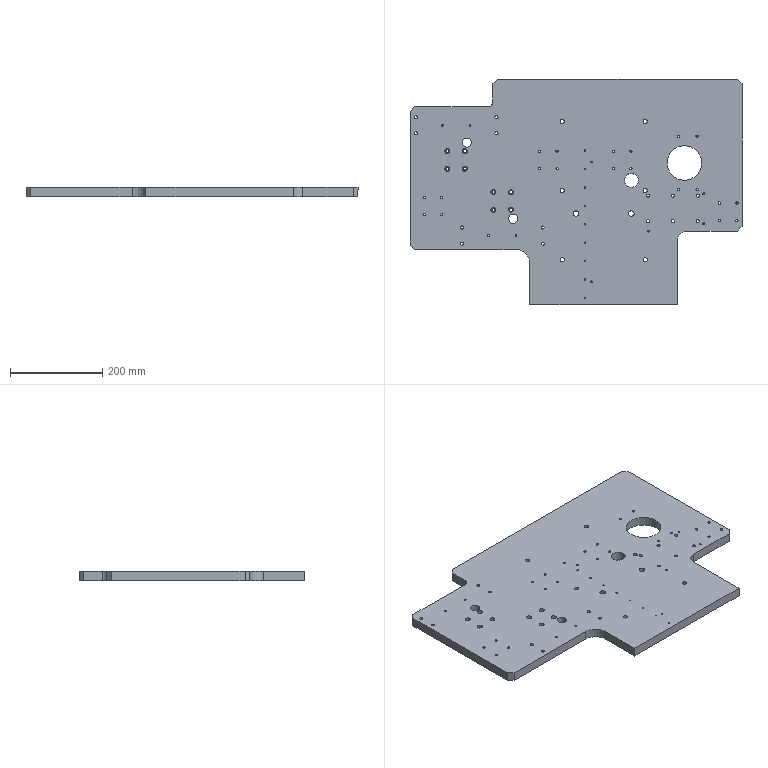Part | SolidWorks | features Cut 8, HoleWzd 8, Chamfer 3, Extrusion 1, Fillet 1, ICE 1, LPattern 1 | 1 solid | 214 faces | box 720 x 490 x 20 mm | volume 5604662 mm3 | cylinder 179 | plane 31 | cone 4 | commonest cylinder face diameters 5 x44 6.8 x28 3.3 x18 4 x18 6.6 x16 11 x16